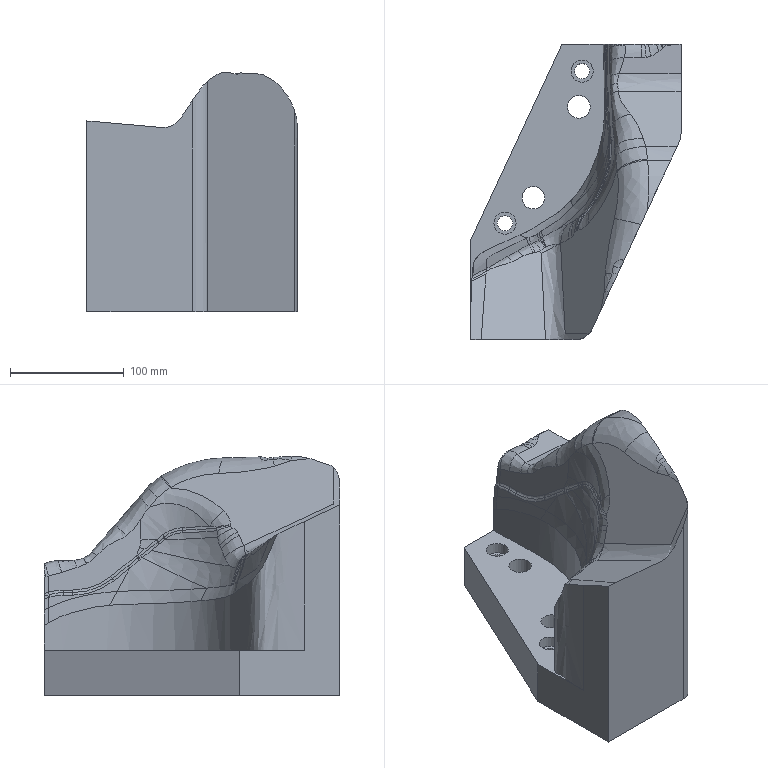Part | NX | features solid 2 | 1 solid | 129 faces | box 185 x 260.001 x 210.738 mm | volume 3824619 mm3 | spline 111 | plane 10 | cylinder 8 | commonest cylinder face diameters 13.5 x2 19.5 x2 20 x2 30 x1 40 x1